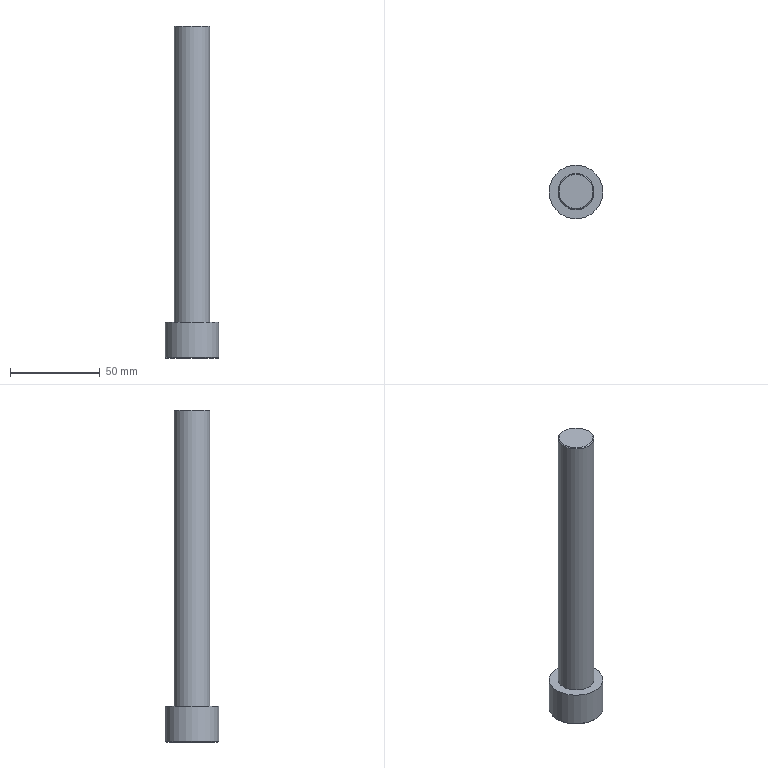Part | NX | features DT 2 | 1 solid | 20 faces | box 30 x 30 x 185 mm | volume 63350 mm3 | plane 15 | cone 3 | cylinder 2 | commonest cylinder face diameters 20 x1 30 x1
STEP:
#1=CARTESIAN_POINT('',(2879.5,-636.815,-40.));
#2=VERTEX_POINT('',#1);
#3=CARTESIAN_POINT('',(2871.,-631.907,-40.));
#4=VERTEX_POINT('',#3);
#5=CARTESIAN_POINT('',(2875.25,-634.361,-40.));
#6=DIRECTION('',(-0.866,0.5,0.));
#7=VECTOR('',#6,1000.);
#8=LINE('',#5,#7);
#9=EDGE_CURVE('',#2,#4,#8,.T.);
#10=ORIENTED_EDGE('',*,*,#9,.T.);
#11=CARTESIAN_POINT('',(2879.5,-627.,-40.));
#12=DIRECTION('',(0.,0.,1.));
#13=DIRECTION('',(-1.,0.,0.));
#14=AXIS2_PLACEMENT_3D('',#11,#12,#13);
#15=CIRCLE('',#14,9.815);
#16=EDGE_CURVE('',#4,#2,#15,.T.);
#17=ORIENTED_EDGE('',*,*,#16,.T.);
#18=EDGE_LOOP('',(#10,#17));
#19=FACE_BOUND('',#18,.T.);
#20=CARTESIAN_POINT('',(2879.5,-627.,-40.));
#21=DIRECTION('',(0.,0.,-1.));
#22=DIRECTION('',(1.,0.,0.));
#23=AXIS2_PLACEMENT_3D('',#20,#21,#22);
#24=PLANE('',#23);
#25=ADVANCED_FACE('',(#19),#24,.F.);
#26=CARTESIAN_POINT('',(2871.,-622.093,-40.));
#27=VERTEX_POINT('',#26);
#28=CARTESIAN_POINT('',(2871.,-627.,-40.));
#29=DIRECTION('',(0.,1.,0.));
#30=VECTOR('',#29,1000.);
#31=LINE('',#28,#30);
#32=EDGE_CURVE('',#4,#27,#31,.T.);
#33=ORIENTED_EDGE('',*,*,#32,.T.);
#34=CARTESIAN_POINT('',(2879.5,-627.,-40.));
#35=DIRECTION('',(0.,0.,1.));
#36=DIRECTION('',(-1.,0.,0.));
#37=AXIS2_PLACEMENT_3D('',#34,#35,#36);
#38=CIRCLE('',#37,9.815);
#39=EDGE_CURVE('',#27,#4,#38,.T.);
#40=ORIENTED_EDGE('',*,*,#39,.T.);
#41=EDGE_LOOP('',(#33,#40));
#42=FACE_BOUND('',#41,.T.);
#43=CARTESIAN_POINT('',(2879.5,-627.,-40.));
#44=DIRECTION('',(0.,0.,-1.));
#45=DIRECTION('',(1.,0.,0.));
#46=AXIS2_PLACEMENT_3D('',#43,#44,#45);
#47=PLANE('',#46);
#48=ADVANCED_FACE('',(#42),#47,.F.);
#49=CARTESIAN_POINT('',(2879.5,-617.185,-40.));
#50=VERTEX_POINT('',#49);
#51=CARTESIAN_POINT('',(2875.25,-619.639,-40.));
#52=DIRECTION('',(0.866,0.5,0.));
#53=VECTOR('',#52,1000.);
#54=LINE('',#51,#53);
#55=EDGE_CURVE('',#27,#50,#54,.T.);
#56=ORIENTED_EDGE('',*,*,#55,.T.);
#57=CARTESIAN_POINT('',(2879.5,-627.,-40.));
#58=DIRECTION('',(0.,0.,1.));
#59=DIRECTION('',(-1.,0.,0.));
#60=AXIS2_PLACEMENT_3D('',#57,#58,#59);
#61=CIRCLE('',#60,9.815);
#62=EDGE_CURVE('',#50,#27,#61,.T.);
#63=ORIENTED_EDGE('',*,*,#62,.T.);
#64=EDGE_LOOP('',(#56,#63));
#65=FACE_BOUND('',#64,.T.);
#66=CARTESIAN_POINT('',(2879.5,-627.,-40.));
#67=DIRECTION('',(0.,0.,-1.));
#68=DIRECTION('',(1.,0.,0.));
#69=AXIS2_PLACEMENT_3D('',#66,#67,#68);
#70=PLANE('',#69);
#71=ADVANCED_FACE('',(#65),#70,.F.);
#72=CARTESIAN_POINT('',(2888.,-622.093,-40.));
#73=VERTEX_POINT('',#72);
#74=CARTESIAN_POINT('',(2883.75,-619.639,-40.));
#75=DIRECTION('',(0.866,-0.5,0.));
#76=VECTOR('',#75,1000.);
#77=LINE('',#74,#76);
#78=EDGE_CURVE('',#50,#73,#77,.T.);
#79=ORIENTED_EDGE('',*,*,#78,.T.);
#80=CARTESIAN_POINT('',(2879.5,-627.,-40.));
#81=DIRECTION('',(0.,0.,1.));
#82=DIRECTION('',(-1.,0.,0.));
#83=AXIS2_PLACEMENT_3D('',#80,#81,#82);
#84=CIRCLE('',#83,9.815);
#85=EDGE_CURVE('',#73,#50,#84,.T.);
#86=ORIENTED_EDGE('',*,*,#85,.T.);
#87=EDGE_LOOP('',(#79,#86));
#88=FACE_BOUND('',#87,.T.);
#89=CARTESIAN_POINT('',(2879.5,-627.,-40.));
#90=DIRECTION('',(0.,0.,-1.));
#91=DIRECTION('',(1.,0.,0.));
#92=AXIS2_PLACEMENT_3D('',#89,#90,#91);
#93=PLANE('',#92);
#94=ADVANCED_FACE('',(#88),#93,.F.);
#95=CARTESIAN_POINT('',(2888.,-631.907,-40.));
#96=VERTEX_POINT('',#95);
#97=CARTESIAN_POINT('',(2888.,-627.,-40.));
#98=DIRECTION('',(0.,-1.,0.));
#99=VECTOR('',#98,1000.);
#100=LINE('',#97,#99);
#101=EDGE_CURVE('',#73,#96,#100,.T.);
#102=ORIENTED_EDGE('',*,*,#101,.T.);
#103=CARTESIAN_POINT('',(2879.5,-627.,-40.));
#104=DIRECTION('',(0.,0.,1.));
#105=DIRECTION('',(-1.,0.,0.));
#106=AXIS2_PLACEMENT_3D('',#103,#104,#105);
#107=CIRCLE('',#106,9.815);
#108=EDGE_CURVE('',#96,#73,#107,.T.);
#109=ORIENTED_EDGE('',*,*,#108,.T.);
#110=EDGE_LOOP('',(#102,#109));
#111=FACE_BOUND('',#110,.T.);
#112=CARTESIAN_POINT('',(2879.5,-627.,-40.));
#113=DIRECTION('',(0.,0.,-1.));
#114=DIRECTION('',(1.,0.,0.));
#115=AXIS2_PLACEMENT_3D('',#112,#113,#114);
#116=PLANE('',#115);
#117=ADVANCED_FACE('',(#111),#116,.F.);
#118=CARTESIAN_POINT('',(2883.75,-634.361,-40.));
#119=DIRECTION('',(-0.866,-0.5,0.));
#120=VECTOR('',#119,1000.);
#121=LINE('',#118,#120);
#122=EDGE_CURVE('',#96,#2,#121,.T.);
#123=ORIENTED_EDGE('',*,*,#122,.T.);
#124=CARTESIAN_POINT('',(2879.5,-627.,-40.));
#125=DIRECTION('',(0.,0.,1.));
#126=DIRECTION('',(-1.,0.,0.));
#127=AXIS2_PLACEMENT_3D('',#124,#125,#126);
#128=CIRCLE('',#127,9.815);
#129=EDGE_CURVE('',#2,#96,#128,.T.);
#130=ORIENTED_EDGE('',*,*,#129,.T.);
#131=EDGE_LOOP('',(#123,#130));
#132=FACE_BOUND('',#131,.T.);
#133=CARTESIAN_POINT('',(2879.5,-627.,-40.));
#134=DIRECTION('',(0.,0.,-1.));
#135=DIRECTION('',(1.,0.,0.));
#136=AXIS2_PLACEMENT_3D('',#133,#134,#135);
#137=PLANE('',#136);
#138=ADVANCED_FACE('',(#132),#137,.F.);
#139=ORIENTED_EDGE('',*,*,#39,.F.);
#140=ORIENTED_EDGE('',*,*,#62,.F.);
#141=ORIENTED_EDGE('',*,*,#85,.F.);
#142=ORIENTED_EDGE('',*,*,#108,.F.);
#143=ORIENTED_EDGE('',*,*,#129,.F.);
#144=ORIENTED_EDGE('',*,*,#16,.F.);
#145=EDGE_LOOP('',(#139,#140,#141,#142,#143,#144));
#146=FACE_BOUND('',#145,.T.);
#147=CARTESIAN_POINT('',(2879.5,-627.,-39.));
#148=VERTEX_POINT('',#147);
#149=VERTEX_LOOP('',#148);
#150=FACE_BOUND('',#149,.T.);
#151=CARTESIAN_POINT('',(2879.5,-627.,-39.5));
#152=DIRECTION('',(0.,0.,-1.));
#153=DIRECTION('',(-1.,0.,0.));
#154=AXIS2_PLACEMENT_3D('',#151,#152,#153);
#155=CONICAL_SURFACE('',#154,4.907,1.469);
#156=ADVANCED_FACE('',(#146,#150),#155,.F.);
#157=CARTESIAN_POINT('',(2879.5,-636.815,-50.));
#158=VERTEX_POINT('',#157);
#159=CARTESIAN_POINT('',(2879.5,-636.815,-45.));
#160=DIRECTION('',(0.,0.,-1.));
#161=VECTOR('',#160,1000.);
#162=LINE('',#159,#161);
#163=EDGE_CURVE('',#2,#158,#162,.T.);
#164=ORIENTED_EDGE('',*,*,#163,.T.);
#165=CARTESIAN_POINT('',(2871.,-631.907,-50.));
#166=VERTEX_POINT('',#165);
#167=CARTESIAN_POINT('',(2875.25,-634.361,-50.));
#168=DIRECTION('',(-0.866,0.5,0.));
#169=VECTOR('',#168,1000.);
#170=LINE('',#167,#169);
#171=EDGE_CURVE('',#158,#166,#170,.T.);
#172=ORIENTED_EDGE('',*,*,#171,.T.);
#173=CARTESIAN_POINT('',(2871.,-631.907,-45.));
#174=DIRECTION('',(0.,0.,-1.));
#175=VECTOR('',#174,1000.);
#176=LINE('',#173,#175);
#177=EDGE_CURVE('',#4,#166,#176,.T.);
#178=ORIENTED_EDGE('',*,*,#177,.F.);
#179=ORIENTED_EDGE('',*,*,#9,.F.);
#180=EDGE_LOOP('',(#164,#172,#178,#179));
#181=FACE_BOUND('',#180,.T.);
#182=CARTESIAN_POINT('',(2875.25,-634.361,-45.));
#183=DIRECTION('',(0.5,0.866,0.));
#184=DIRECTION('',(0.,0.,1.));
#185=AXIS2_PLACEMENT_3D('',#182,#183,#184);
#186=PLANE('',#185);
#187=ADVANCED_FACE('',(#181),#186,.T.);
#188=CARTESIAN_POINT('',(2888.,-631.907,-50.));
#189=VERTEX_POINT('',#188);
#190=CARTESIAN_POINT('',(2888.,-631.907,-45.));
#191=DIRECTION('',(0.,0.,-1.));
#192=VECTOR('',#191,1000.);
#193=LINE('',#190,#192);
#194=EDGE_CURVE('',#96,#189,#193,.T.);
#195=ORIENTED_EDGE('',*,*,#194,.T.);
#196=CARTESIAN_POINT('',(2883.75,-634.361,-50.));
#197=DIRECTION('',(-0.866,-0.5,0.));
#198=VECTOR('',#197,1000.);
#199=LINE('',#196,#198);
#200=EDGE_CURVE('',#189,#158,#199,.T.);
#201=ORIENTED_EDGE('',*,*,#200,.T.);
#202=ORIENTED_EDGE('',*,*,#163,.F.);
#203=ORIENTED_EDGE('',*,*,#122,.F.);
#204=EDGE_LOOP('',(#195,#201,#202,#203));
#205=FACE_BOUND('',#204,.T.);
#206=CARTESIAN_POINT('',(2883.75,-634.361,-45.));
#207=DIRECTION('',(-0.5,0.866,0.));
#208=DIRECTION('',(0.,0.,-1.));
#209=AXIS2_PLACEMENT_3D('',#206,#207,#208);
#210=PLANE('',#209);
#211=ADVANCED_FACE('',(#205),#210,.T.);
#212=CARTESIAN_POINT('',(2888.,-622.093,-50.));
#213=VERTEX_POINT('',#212);
#214=CARTESIAN_POINT('',(2888.,-622.093,-45.));
#215=DIRECTION('',(0.,0.,-1.));
#216=VECTOR('',#215,1000.);
#217=LINE('',#214,#216);
#218=EDGE_CURVE('',#73,#213,#217,.T.);
#219=ORIENTED_EDGE('',*,*,#218,.T.);
#220=CARTESIAN_POINT('',(2888.,-627.,-50.));
#221=DIRECTION('',(0.,-1.,0.));
#222=VECTOR('',#221,1000.);
#223=LINE('',#220,#222);
#224=EDGE_CURVE('',#213,#189,#223,.T.);
#225=ORIENTED_EDGE('',*,*,#224,.T.);
#226=ORIENTED_EDGE('',*,*,#194,.F.);
#227=ORIENTED_EDGE('',*,*,#101,.F.);
#228=EDGE_LOOP('',(#219,#225,#226,#227));
#229=FACE_BOUND('',#228,.T.);
#230=CARTESIAN_POINT('',(2888.,-627.,-45.));
#231=DIRECTION('',(-1.,0.,0.));
#232=DIRECTION('',(0.,0.,-1.));
#233=AXIS2_PLACEMENT_3D('',#230,#231,#232);
#234=PLANE('',#233);
#235=ADVANCED_FACE('',(#229),#234,.T.);
#236=CARTESIAN_POINT('',(2879.5,-617.185,-50.));
#237=VERTEX_POINT('',#236);
#238=CARTESIAN_POINT('',(2879.5,-617.185,-45.));
#239=DIRECTION('',(0.,0.,-1.));
#240=VECTOR('',#239,1000.);
#241=LINE('',#238,#240);
#242=EDGE_CURVE('',#50,#237,#241,.T.);
#243=ORIENTED_EDGE('',*,*,#242,.T.);
#244=CARTESIAN_POINT('',(2883.75,-619.639,-50.));
#245=DIRECTION('',(0.866,-0.5,0.));
#246=VECTOR('',#245,1000.);
#247=LINE('',#244,#246);
#248=EDGE_CURVE('',#237,#213,#247,.T.);
#249=ORIENTED_EDGE('',*,*,#248,.T.);
#250=ORIENTED_EDGE('',*,*,#218,.F.);
#251=ORIENTED_EDGE('',*,*,#78,.F.);
#252=EDGE_LOOP('',(#243,#249,#250,#251));
#253=FACE_BOUND('',#252,.T.);
#254=CARTESIAN_POINT('',(2883.75,-619.639,-45.));
#255=DIRECTION('',(-0.5,-0.866,0.));
#256=DIRECTION('',(0.,0.,-1.));
#257=AXIS2_PLACEMENT_3D('',#254,#255,#256);
#258=PLANE('',#257);
#259=ADVANCED_FACE('',(#253),#258,.T.);
#260=CARTESIAN_POINT('',(2871.,-622.093,-50.));
#261=VERTEX_POINT('',#260);
#262=CARTESIAN_POINT('',(2871.,-622.093,-45.));
#263=DIRECTION('',(0.,0.,-1.));
#264=VECTOR('',#263,1000.);
#265=LINE('',#262,#264);
#266=EDGE_CURVE('',#27,#261,#265,.T.);
#267=ORIENTED_EDGE('',*,*,#266,.T.);
#268=CARTESIAN_POINT('',(2875.25,-619.639,-50.));
#269=DIRECTION('',(0.866,0.5,0.));
#270=VECTOR('',#269,1000.);
#271=LINE('',#268,#270);
#272=EDGE_CURVE('',#261,#237,#271,.T.);
#273=ORIENTED_EDGE('',*,*,#272,.T.);
#274=ORIENTED_EDGE('',*,*,#242,.F.);
#275=ORIENTED_EDGE('',*,*,#55,.F.);
#276=EDGE_LOOP('',(#267,#273,#274,#275));
#277=FACE_BOUND('',#276,.T.);
#278=CARTESIAN_POINT('',(2875.25,-619.639,-45.));
#279=DIRECTION('',(0.5,-0.866,0.));
#280=DIRECTION('',(0.,0.,1.));
#281=AXIS2_PLACEMENT_3D('',#278,#279,#280);
#282=PLANE('',#281);
#283=ADVANCED_FACE('',(#277),#282,.T.);
#284=ORIENTED_EDGE('',*,*,#177,.T.);
#285=CARTESIAN_POINT('',(2871.,-627.,-50.));
#286=DIRECTION('',(0.,1.,0.));
#287=VECTOR('',#286,1000.);
#288=LINE('',#285,#287);
#289=EDGE_CURVE('',#166,#261,#288,.T.);
#290=ORIENTED_EDGE('',*,*,#289,.T.);
#291=ORIENTED_EDGE('',*,*,#266,.F.);
#292=ORIENTED_EDGE('',*,*,#32,.F.);
#293=EDGE_LOOP('',(#284,#290,#291,#292));
#294=FACE_BOUND('',#293,.T.);
#295=CARTESIAN_POINT('',(2871.,-627.,-45.));
#296=DIRECTION('',(1.,0.,0.));
#297=DIRECTION('',(0.,0.,1.));
#298=AXIS2_PLACEMENT_3D('',#295,#296,#297);
#299=PLANE('',#298);
#300=ADVANCED_FACE('',(#294),#299,.T.);
#301=CARTESIAN_POINT('',(2869.5,-627.,134.5));
#302=VERTEX_POINT('',#301);
#303=CARTESIAN_POINT('',(2879.5,-627.,134.5));
#304=DIRECTION('',(0.,0.,-1.));
#305=DIRECTION('',(1.,0.,0.));
#306=AXIS2_PLACEMENT_3D('',#303,#304,#305);
#307=CIRCLE('',#306,10.);
#308=EDGE_CURVE('',#302,#302,#307,.T.);
#309=ORIENTED_EDGE('',*,*,#308,.F.);
#310=EDGE_LOOP('',(#309));
#311=FACE_BOUND('',#310,.T.);
#312=CARTESIAN_POINT('',(2870.,-627.,135.));
#313=VERTEX_POINT('',#312);
#314=CARTESIAN_POINT('',(2879.5,-627.,135.));
#315=DIRECTION('',(0.,0.,1.));
#316=DIRECTION('',(1.,0.,0.));
#317=AXIS2_PLACEMENT_3D('',#314,#315,#316);
#318=CIRCLE('',#317,9.5);
#319=EDGE_CURVE('',#313,#313,#318,.T.);
#320=ORIENTED_EDGE('',*,*,#319,.F.);
#321=EDGE_LOOP('',(#320));
#322=FACE_BOUND('',#321,.T.);
#323=CARTESIAN_POINT('',(2879.5,-627.,135.));
#324=DIRECTION('',(0.,0.,-1.));
#325=DIRECTION('',(1.,0.,0.));
#326=AXIS2_PLACEMENT_3D('',#323,#324,#325);
#327=CONICAL_SURFACE('',#326,9.5,0.7854);
#328=ADVANCED_FACE('',(#311,#322),#327,.T.);
#329=CARTESIAN_POINT('',(2869.5,-627.,-30.));
#330=VERTEX_POINT('',#329);
#331=CARTESIAN_POINT('',(2879.5,-627.,-30.));
#332=DIRECTION('',(0.,0.,1.));
#333=DIRECTION('',(-1.,0.,0.));
#334=AXIS2_PLACEMENT_3D('',#331,#332,#333);
#335=CIRCLE('',#334,10.);
#336=EDGE_CURVE('',#330,#330,#335,.T.);
#337=ORIENTED_EDGE('',*,*,#336,.T.);
#338=EDGE_LOOP('',(#337));
#339=FACE_BOUND('',#338,.T.);
#340=ORIENTED_EDGE('',*,*,#308,.T.);
#341=EDGE_LOOP('',(#340));
#342=FACE_BOUND('',#341,.T.);
#343=CARTESIAN_POINT('',(2879.5,-627.,40.));
#344=DIRECTION('',(0.,0.,1.));
#345=DIRECTION('',(-1.,0.,0.));
#346=AXIS2_PLACEMENT_3D('',#343,#344,#345);
#347=CYLINDRICAL_SURFACE('',#346,10.);
#348=ADVANCED_FACE('',(#339,#342),#347,.T.);
#349=ORIENTED_EDGE('',*,*,#319,.T.);
#350=EDGE_LOOP('',(#349));
#351=FACE_BOUND('',#350,.T.);
#352=CARTESIAN_POINT('',(2879.5,-627.,135.));
#353=DIRECTION('',(0.,0.,1.));
#354=DIRECTION('',(-1.,0.,0.));
#355=AXIS2_PLACEMENT_3D('',#352,#353,#354);
#356=PLANE('',#355);
#357=ADVANCED_FACE('',(#351),#356,.T.);
#358=CARTESIAN_POINT('',(2864.5,-627.,-49.5));
#359=VERTEX_POINT('',#358);
#360=CARTESIAN_POINT('',(2879.5,-627.,-49.5));
#361=DIRECTION('',(0.,0.,1.));
#362=DIRECTION('',(1.,0.,0.));
#363=AXIS2_PLACEMENT_3D('',#360,#361,#362);
#364=CIRCLE('',#363,15.);
#365=EDGE_CURVE('',#359,#359,#364,.T.);
#366=ORIENTED_EDGE('',*,*,#365,.F.);
#367=EDGE_LOOP('',(#366));
#368=FACE_BOUND('',#367,.T.);
#369=CARTESIAN_POINT('',(2865.,-627.,-50.));
#370=VERTEX_POINT('',#369);
#371=CARTESIAN_POINT('',(2879.5,-627.,-50.));
#372=DIRECTION('',(0.,0.,-1.));
#373=DIRECTION('',(1.,0.,0.));
#374=AXIS2_PLACEMENT_3D('',#371,#372,#373);
#375=CIRCLE('',#374,14.5);
#376=EDGE_CURVE('',#370,#370,#375,.T.);
#377=ORIENTED_EDGE('',*,*,#376,.F.);
#378=EDGE_LOOP('',(#377));
#379=FACE_BOUND('',#378,.T.);
#380=CARTESIAN_POINT('',(2879.5,-627.,-50.));
#381=DIRECTION('',(0.,0.,1.));
#382=DIRECTION('',(1.,0.,0.));
#383=AXIS2_PLACEMENT_3D('',#380,#381,#382);
#384=CONICAL_SURFACE('',#383,14.5,0.7854);
#385=ADVANCED_FACE('',(#368,#379),#384,.T.);
#386=CARTESIAN_POINT('',(2864.5,-627.,-30.));
#387=VERTEX_POINT('',#386);
#388=CARTESIAN_POINT('',(2879.5,-627.,-30.));
#389=DIRECTION('',(0.,0.,-1.));
#390=DIRECTION('',(-1.,0.,0.));
#391=AXIS2_PLACEMENT_3D('',#388,#389,#390);
#392=CIRCLE('',#391,15.);
#393=EDGE_CURVE('',#387,#387,#392,.T.);
#394=ORIENTED_EDGE('',*,*,#393,.T.);
#395=EDGE_LOOP('',(#394));
#396=FACE_BOUND('',#395,.T.);
#397=ORIENTED_EDGE('',*,*,#365,.T.);
#398=EDGE_LOOP('',(#397));
#399=FACE_BOUND('',#398,.T.);
#400=CARTESIAN_POINT('',(2879.5,-627.,-40.));
#401=DIRECTION('',(0.,0.,1.));
#402=DIRECTION('',(-1.,0.,0.));
#403=AXIS2_PLACEMENT_3D('',#400,#401,#402);
#404=CYLINDRICAL_SURFACE('',#403,15.);
#405=ADVANCED_FACE('',(#396,#399),#404,.T.);
#406=ORIENTED_EDGE('',*,*,#171,.F.);
#407=ORIENTED_EDGE('',*,*,#200,.F.);
#408=ORIENTED_EDGE('',*,*,#224,.F.);
#409=ORIENTED_EDGE('',*,*,#248,.F.);
#410=ORIENTED_EDGE('',*,*,#272,.F.);
#411=ORIENTED_EDGE('',*,*,#289,.F.);
#412=EDGE_LOOP('',(#406,#407,#408,#409,#410,#411));
#413=FACE_BOUND('',#412,.T.);
#414=ORIENTED_EDGE('',*,*,#376,.T.);
#415=EDGE_LOOP('',(#414));
#416=FACE_BOUND('',#415,.T.);
#417=CARTESIAN_POINT('',(2879.5,-627.,-50.));
#418=DIRECTION('',(0.,0.,-1.));
#419=DIRECTION('',(1.,0.,0.));
#420=AXIS2_PLACEMENT_3D('',#417,#418,#419);
#421=PLANE('',#420);
#422=ADVANCED_FACE('',(#413,#416),#421,.T.);
#423=ORIENTED_EDGE('',*,*,#336,.F.);
#424=EDGE_LOOP('',(#423));
#425=FACE_BOUND('',#424,.T.);
#426=ORIENTED_EDGE('',*,*,#393,.F.);
#427=EDGE_LOOP('',(#426));
#428=FACE_BOUND('',#427,.T.);
#429=CARTESIAN_POINT('',(2879.5,-627.,-30.));
#430=DIRECTION('',(0.,0.,1.));
#431=DIRECTION('',(-1.,0.,0.));
#432=AXIS2_PLACEMENT_3D('',#429,#430,#431);
#433=PLANE('',#432);
#434=ADVANCED_FACE('',(#425,#428),#433,.T.);
#435=CLOSED_SHELL('',(#25,#48,#71,#94,#117,#138,#156,#187,#211,#235,#259,#283,#300,#328,#348,#357,#385,#405,#422,#434));
#436=MANIFOLD_SOLID_BREP('',#435);
#437=(LENGTH_UNIT()NAMED_UNIT(*)SI_UNIT(.MILLI.,.METRE.));
#438=UNCERTAINTY_MEASURE_WITH_UNIT(LENGTH_MEASURE(0.00001),#437,'','');
#439=(NAMED_UNIT(*)PLANE_ANGLE_UNIT()SI_UNIT($,.RADIAN.));
#440=(NAMED_UNIT(*)SI_UNIT($,.STERADIAN.)SOLID_ANGLE_UNIT());
#441=(GEOMETRIC_REPRESENTATION_CONTEXT(3)GLOBAL_UNCERTAINTY_ASSIGNED_CONTEXT((#438))GLOBAL_UNIT_ASSIGNED_CONTEXT((#437,#439,#440))REPRESENTATION_CONTEXT('',''));
#442=ADVANCED_BREP_SHAPE_REPRESENTATION('',(#436),#441);